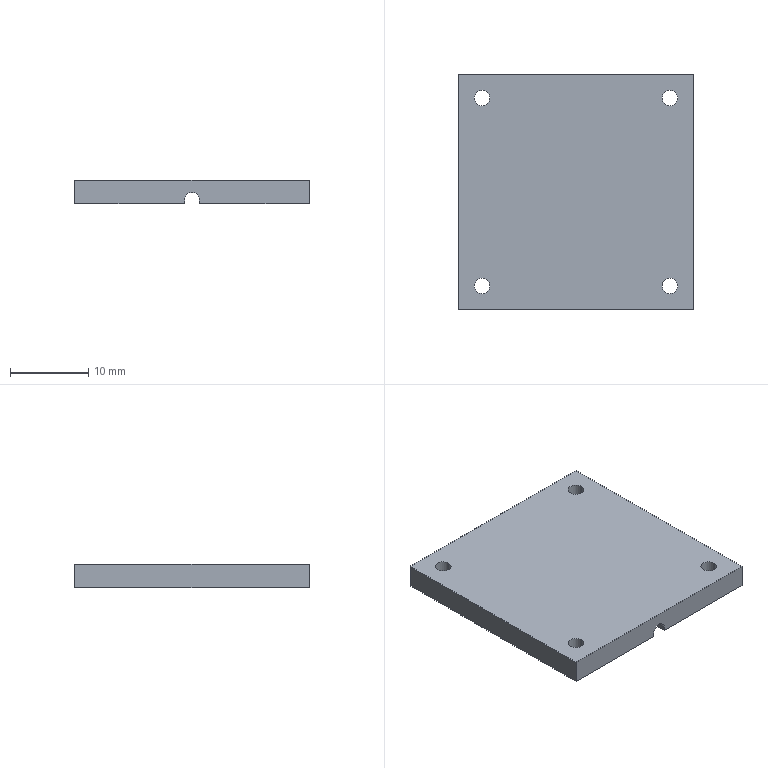Part | SolidWorks | features ICE 2, Extrusion 1 | 1 solid | 18 faces | box 30 x 30 x 3 mm | volume 2591 mm3 | cylinder 9 | plane 9 | commonest cylinder face diameters 2 x8 1.9 x1
STEP:
#1=CARTESIAN_POINT('',(-11.,-12.,0.));
#2=VERTEX_POINT('',#1);
#3=CARTESIAN_POINT('',(-13.,-12.,0.));
#4=VERTEX_POINT('',#3);
#5=CARTESIAN_POINT('',(-12.,-12.,0.));
#6=DIRECTION('',(0.,0.,-1.));
#7=DIRECTION('',(-1.,0.,0.));
#8=AXIS2_PLACEMENT_3D('',#5,#6,#7);
#9=CIRCLE('',#8,1.);
#10=EDGE_CURVE('',#2,#4,#9,.T.);
#11=ORIENTED_EDGE('',*,*,#10,.T.);
#12=CARTESIAN_POINT('',(-13.,-12.,3.));
#13=VERTEX_POINT('',#12);
#14=CARTESIAN_POINT('',(-13.,-12.,-16.));
#15=DIRECTION('',(0.,0.,1.));
#16=VECTOR('',#15,1000.);
#17=LINE('',#14,#16);
#18=EDGE_CURVE('',#4,#13,#17,.T.);
#19=ORIENTED_EDGE('',*,*,#18,.T.);
#20=CARTESIAN_POINT('',(-11.,-12.,3.));
#21=VERTEX_POINT('',#20);
#22=CARTESIAN_POINT('',(-12.,-12.,3.));
#23=DIRECTION('',(0.,0.,1.));
#24=DIRECTION('',(1.,0.,0.));
#25=AXIS2_PLACEMENT_3D('',#22,#23,#24);
#26=CIRCLE('',#25,1.);
#27=EDGE_CURVE('',#13,#21,#26,.T.);
#28=ORIENTED_EDGE('',*,*,#27,.T.);
#29=CARTESIAN_POINT('',(-11.,-12.,-16.));
#30=DIRECTION('',(0.,0.,1.));
#31=VECTOR('',#30,1000.);
#32=LINE('',#29,#31);
#33=EDGE_CURVE('',#2,#21,#32,.T.);
#34=ORIENTED_EDGE('',*,*,#33,.F.);
#35=EDGE_LOOP('',(#11,#19,#28,#34));
#36=FACE_OUTER_BOUND('',#35,.T.);
#37=CARTESIAN_POINT('',(-12.,-12.,-16.));
#38=DIRECTION('',(0.,0.,1.));
#39=DIRECTION('',(1.,0.,0.));
#40=AXIS2_PLACEMENT_3D('',#37,#38,#39);
#41=CYLINDRICAL_SURFACE('',#40,1.);
#42=ADVANCED_FACE('',(#36),#41,.F.);
#43=CARTESIAN_POINT('',(13.,-12.,0.));
#44=VERTEX_POINT('',#43);
#45=CARTESIAN_POINT('',(11.,-12.,0.));
#46=VERTEX_POINT('',#45);
#47=CARTESIAN_POINT('',(12.,-12.,0.));
#48=DIRECTION('',(0.,0.,-1.));
#49=DIRECTION('',(-1.,0.,0.));
#50=AXIS2_PLACEMENT_3D('',#47,#48,#49);
#51=CIRCLE('',#50,1.);
#52=EDGE_CURVE('',#44,#46,#51,.T.);
#53=ORIENTED_EDGE('',*,*,#52,.T.);
#54=CARTESIAN_POINT('',(11.,-12.,3.));
#55=VERTEX_POINT('',#54);
#56=CARTESIAN_POINT('',(11.,-12.,-16.));
#57=DIRECTION('',(0.,0.,1.));
#58=VECTOR('',#57,1000.);
#59=LINE('',#56,#58);
#60=EDGE_CURVE('',#46,#55,#59,.T.);
#61=ORIENTED_EDGE('',*,*,#60,.T.);
#62=CARTESIAN_POINT('',(13.,-12.,3.));
#63=VERTEX_POINT('',#62);
#64=CARTESIAN_POINT('',(12.,-12.,3.));
#65=DIRECTION('',(0.,0.,1.));
#66=DIRECTION('',(1.,0.,0.));
#67=AXIS2_PLACEMENT_3D('',#64,#65,#66);
#68=CIRCLE('',#67,1.);
#69=EDGE_CURVE('',#55,#63,#68,.T.);
#70=ORIENTED_EDGE('',*,*,#69,.T.);
#71=CARTESIAN_POINT('',(13.,-12.,-16.));
#72=DIRECTION('',(0.,0.,1.));
#73=VECTOR('',#72,1000.);
#74=LINE('',#71,#73);
#75=EDGE_CURVE('',#44,#63,#74,.T.);
#76=ORIENTED_EDGE('',*,*,#75,.F.);
#77=EDGE_LOOP('',(#53,#61,#70,#76));
#78=FACE_OUTER_BOUND('',#77,.T.);
#79=CARTESIAN_POINT('',(12.,-12.,-16.));
#80=DIRECTION('',(0.,0.,1.));
#81=DIRECTION('',(1.,0.,0.));
#82=AXIS2_PLACEMENT_3D('',#79,#80,#81);
#83=CYLINDRICAL_SURFACE('',#82,1.);
#84=ADVANCED_FACE('',(#78),#83,.F.);
#85=CARTESIAN_POINT('',(13.,12.,0.));
#86=VERTEX_POINT('',#85);
#87=CARTESIAN_POINT('',(11.,12.,0.));
#88=VERTEX_POINT('',#87);
#89=CARTESIAN_POINT('',(12.,12.,0.));
#90=DIRECTION('',(0.,0.,-1.));
#91=DIRECTION('',(-1.,0.,0.));
#92=AXIS2_PLACEMENT_3D('',#89,#90,#91);
#93=CIRCLE('',#92,1.);
#94=EDGE_CURVE('',#86,#88,#93,.T.);
#95=ORIENTED_EDGE('',*,*,#94,.T.);
#96=CARTESIAN_POINT('',(11.,12.,3.));
#97=VERTEX_POINT('',#96);
#98=CARTESIAN_POINT('',(11.,12.,-16.));
#99=DIRECTION('',(0.,0.,1.));
#100=VECTOR('',#99,1000.);
#101=LINE('',#98,#100);
#102=EDGE_CURVE('',#88,#97,#101,.T.);
#103=ORIENTED_EDGE('',*,*,#102,.T.);
#104=CARTESIAN_POINT('',(13.,12.,3.));
#105=VERTEX_POINT('',#104);
#106=CARTESIAN_POINT('',(12.,12.,3.));
#107=DIRECTION('',(0.,0.,1.));
#108=DIRECTION('',(1.,0.,0.));
#109=AXIS2_PLACEMENT_3D('',#106,#107,#108);
#110=CIRCLE('',#109,1.);
#111=EDGE_CURVE('',#97,#105,#110,.T.);
#112=ORIENTED_EDGE('',*,*,#111,.T.);
#113=CARTESIAN_POINT('',(13.,12.,-16.));
#114=DIRECTION('',(0.,0.,1.));
#115=VECTOR('',#114,1000.);
#116=LINE('',#113,#115);
#117=EDGE_CURVE('',#86,#105,#116,.T.);
#118=ORIENTED_EDGE('',*,*,#117,.F.);
#119=EDGE_LOOP('',(#95,#103,#112,#118));
#120=FACE_OUTER_BOUND('',#119,.T.);
#121=CARTESIAN_POINT('',(12.,12.,-16.));
#122=DIRECTION('',(0.,0.,1.));
#123=DIRECTION('',(1.,0.,0.));
#124=AXIS2_PLACEMENT_3D('',#121,#122,#123);
#125=CYLINDRICAL_SURFACE('',#124,1.);
#126=ADVANCED_FACE('',(#120),#125,.F.);
#127=CARTESIAN_POINT('',(-11.,12.,0.));
#128=VERTEX_POINT('',#127);
#129=CARTESIAN_POINT('',(-13.,12.,0.));
#130=VERTEX_POINT('',#129);
#131=CARTESIAN_POINT('',(-12.,12.,0.));
#132=DIRECTION('',(0.,0.,-1.));
#133=DIRECTION('',(-1.,0.,0.));
#134=AXIS2_PLACEMENT_3D('',#131,#132,#133);
#135=CIRCLE('',#134,1.);
#136=EDGE_CURVE('',#128,#130,#135,.T.);
#137=ORIENTED_EDGE('',*,*,#136,.T.);
#138=CARTESIAN_POINT('',(-13.,12.,3.));
#139=VERTEX_POINT('',#138);
#140=CARTESIAN_POINT('',(-13.,12.,-16.));
#141=DIRECTION('',(0.,0.,1.));
#142=VECTOR('',#141,1000.);
#143=LINE('',#140,#142);
#144=EDGE_CURVE('',#130,#139,#143,.T.);
#145=ORIENTED_EDGE('',*,*,#144,.T.);
#146=CARTESIAN_POINT('',(-11.,12.,3.));
#147=VERTEX_POINT('',#146);
#148=CARTESIAN_POINT('',(-12.,12.,3.));
#149=DIRECTION('',(0.,0.,1.));
#150=DIRECTION('',(1.,0.,0.));
#151=AXIS2_PLACEMENT_3D('',#148,#149,#150);
#152=CIRCLE('',#151,1.);
#153=EDGE_CURVE('',#139,#147,#152,.T.);
#154=ORIENTED_EDGE('',*,*,#153,.T.);
#155=CARTESIAN_POINT('',(-11.,12.,-16.));
#156=DIRECTION('',(0.,0.,1.));
#157=VECTOR('',#156,1000.);
#158=LINE('',#155,#157);
#159=EDGE_CURVE('',#128,#147,#158,.T.);
#160=ORIENTED_EDGE('',*,*,#159,.F.);
#161=EDGE_LOOP('',(#137,#145,#154,#160));
#162=FACE_OUTER_BOUND('',#161,.T.);
#163=CARTESIAN_POINT('',(-12.,12.,-16.));
#164=DIRECTION('',(0.,0.,1.));
#165=DIRECTION('',(1.,0.,0.));
#166=AXIS2_PLACEMENT_3D('',#163,#164,#165);
#167=CYLINDRICAL_SURFACE('',#166,1.);
#168=ADVANCED_FACE('',(#162),#167,.F.);
#169=CARTESIAN_POINT('',(0.95,15.,0.));
#170=VERTEX_POINT('',#169);
#171=CARTESIAN_POINT('',(0.95,-15.,0.));
#172=VERTEX_POINT('',#171);
#173=CARTESIAN_POINT('',(0.95,0.,0.));
#174=DIRECTION('',(0.,-1.,0.));
#175=VECTOR('',#174,1000.);
#176=LINE('',#173,#175);
#177=EDGE_CURVE('',#170,#172,#176,.T.);
#178=ORIENTED_EDGE('',*,*,#177,.F.);
#179=CARTESIAN_POINT('',(15.,15.,0.));
#180=VERTEX_POINT('',#179);
#181=CARTESIAN_POINT('',(-15.,15.,0.));
#182=DIRECTION('',(-1.,0.,0.));
#183=VECTOR('',#182,1000.);
#184=LINE('',#181,#183);
#185=EDGE_CURVE('',#180,#170,#184,.T.);
#186=ORIENTED_EDGE('',*,*,#185,.F.);
#187=CARTESIAN_POINT('',(15.,-15.,0.));
#188=VERTEX_POINT('',#187);
#189=CARTESIAN_POINT('',(15.,-15.,0.));
#190=DIRECTION('',(0.,1.,0.));
#191=VECTOR('',#190,1000.);
#192=LINE('',#189,#191);
#193=EDGE_CURVE('',#188,#180,#192,.T.);
#194=ORIENTED_EDGE('',*,*,#193,.F.);
#195=CARTESIAN_POINT('',(-15.,-15.,0.));
#196=DIRECTION('',(1.,0.,0.));
#197=VECTOR('',#196,1000.);
#198=LINE('',#195,#197);
#199=EDGE_CURVE('',#172,#188,#198,.T.);
#200=ORIENTED_EDGE('',*,*,#199,.F.);
#201=EDGE_LOOP('',(#178,#186,#194,#200));
#202=FACE_OUTER_BOUND('',#201,.T.);
#203=ORIENTED_EDGE('',*,*,#94,.F.);
#204=CARTESIAN_POINT('',(12.,12.,0.));
#205=DIRECTION('',(0.,0.,-1.));
#206=DIRECTION('',(-1.,0.,0.));
#207=AXIS2_PLACEMENT_3D('',#204,#205,#206);
#208=CIRCLE('',#207,1.);
#209=EDGE_CURVE('',#88,#86,#208,.T.);
#210=ORIENTED_EDGE('',*,*,#209,.F.);
#211=EDGE_LOOP('',(#203,#210));
#212=FACE_BOUND('',#211,.T.);
#213=ORIENTED_EDGE('',*,*,#52,.F.);
#214=CARTESIAN_POINT('',(12.,-12.,0.));
#215=DIRECTION('',(0.,0.,-1.));
#216=DIRECTION('',(-1.,0.,0.));
#217=AXIS2_PLACEMENT_3D('',#214,#215,#216);
#218=CIRCLE('',#217,1.);
#219=EDGE_CURVE('',#46,#44,#218,.T.);
#220=ORIENTED_EDGE('',*,*,#219,.F.);
#221=EDGE_LOOP('',(#213,#220));
#222=FACE_BOUND('',#221,.T.);
#223=CARTESIAN_POINT('',(0.,0.,0.));
#224=DIRECTION('',(0.,0.,-1.));
#225=DIRECTION('',(-1.,0.,0.));
#226=AXIS2_PLACEMENT_3D('',#223,#224,#225);
#227=PLANE('',#226);
#228=ADVANCED_FACE('',(#202,#212,#222),#227,.T.);
#229=ORIENTED_EDGE('',*,*,#193,.T.);
#230=CARTESIAN_POINT('',(15.,15.,3.));
#231=VERTEX_POINT('',#230);
#232=CARTESIAN_POINT('',(15.,15.,3.));
#233=DIRECTION('',(0.,0.,-1.));
#234=VECTOR('',#233,1000.);
#235=LINE('',#232,#234);
#236=EDGE_CURVE('',#231,#180,#235,.T.);
#237=ORIENTED_EDGE('',*,*,#236,.F.);
#238=CARTESIAN_POINT('',(15.,-15.,3.));
#239=VERTEX_POINT('',#238);
#240=CARTESIAN_POINT('',(15.,-15.,3.));
#241=DIRECTION('',(0.,1.,0.));
#242=VECTOR('',#241,1000.);
#243=LINE('',#240,#242);
#244=EDGE_CURVE('',#239,#231,#243,.T.);
#245=ORIENTED_EDGE('',*,*,#244,.F.);
#246=CARTESIAN_POINT('',(15.,-15.,3.));
#247=DIRECTION('',(0.,0.,-1.));
#248=VECTOR('',#247,1000.);
#249=LINE('',#246,#248);
#250=EDGE_CURVE('',#239,#188,#249,.T.);
#251=ORIENTED_EDGE('',*,*,#250,.T.);
#252=EDGE_LOOP('',(#229,#237,#245,#251));
#253=FACE_OUTER_BOUND('',#252,.T.);
#254=CARTESIAN_POINT('',(15.,-15.,3.));
#255=DIRECTION('',(-1.,0.,0.));
#256=DIRECTION('',(0.,0.,1.));
#257=AXIS2_PLACEMENT_3D('',#254,#255,#256);
#258=PLANE('',#257);
#259=ADVANCED_FACE('',(#253),#258,.F.);
#260=ORIENTED_EDGE('',*,*,#185,.T.);
#261=CARTESIAN_POINT('',(0.95,15.,0.5));
#262=VERTEX_POINT('',#261);
#263=CARTESIAN_POINT('',(0.95,15.,3.));
#264=DIRECTION('',(0.,0.,1.));
#265=VECTOR('',#264,1000.);
#266=LINE('',#263,#265);
#267=EDGE_CURVE('',#170,#262,#266,.T.);
#268=ORIENTED_EDGE('',*,*,#267,.T.);
#269=CARTESIAN_POINT('',(-0.95,15.,0.5));
#270=VERTEX_POINT('',#269);
#271=CARTESIAN_POINT('',(0.,15.,0.5));
#272=DIRECTION('',(0.,-1.,0.));
#273=DIRECTION('',(0.,0.,-1.));
#274=AXIS2_PLACEMENT_3D('',#271,#272,#273);
#275=CIRCLE('',#274,0.95);
#276=EDGE_CURVE('',#262,#270,#275,.T.);
#277=ORIENTED_EDGE('',*,*,#276,.T.);
#278=CARTESIAN_POINT('',(-0.95,15.,0.));
#279=VERTEX_POINT('',#278);
#280=CARTESIAN_POINT('',(-0.95,15.,3.));
#281=DIRECTION('',(0.,0.,-1.));
#282=VECTOR('',#281,1000.);
#283=LINE('',#280,#282);
#284=EDGE_CURVE('',#270,#279,#283,.T.);
#285=ORIENTED_EDGE('',*,*,#284,.T.);
#286=CARTESIAN_POINT('',(-15.,15.,0.));
#287=VERTEX_POINT('',#286);
#288=CARTESIAN_POINT('',(-15.,15.,0.));
#289=DIRECTION('',(-1.,0.,0.));
#290=VECTOR('',#289,1000.);
#291=LINE('',#288,#290);
#292=EDGE_CURVE('',#279,#287,#291,.T.);
#293=ORIENTED_EDGE('',*,*,#292,.T.);
#294=CARTESIAN_POINT('',(-15.,15.,3.));
#295=VERTEX_POINT('',#294);
#296=CARTESIAN_POINT('',(-15.,15.,3.));
#297=DIRECTION('',(0.,0.,-1.));
#298=VECTOR('',#297,1000.);
#299=LINE('',#296,#298);
#300=EDGE_CURVE('',#295,#287,#299,.T.);
#301=ORIENTED_EDGE('',*,*,#300,.F.);
#302=CARTESIAN_POINT('',(-15.,15.,3.));
#303=DIRECTION('',(-1.,0.,0.));
#304=VECTOR('',#303,1000.);
#305=LINE('',#302,#304);
#306=EDGE_CURVE('',#231,#295,#305,.T.);
#307=ORIENTED_EDGE('',*,*,#306,.F.);
#308=ORIENTED_EDGE('',*,*,#236,.T.);
#309=EDGE_LOOP('',(#260,#268,#277,#285,#293,#301,#307,#308));
#310=FACE_OUTER_BOUND('',#309,.T.);
#311=CARTESIAN_POINT('',(-15.,15.,3.));
#312=DIRECTION('',(0.,-1.,0.));
#313=DIRECTION('',(0.,0.,-1.));
#314=AXIS2_PLACEMENT_3D('',#311,#312,#313);
#315=PLANE('',#314);
#316=ADVANCED_FACE('',(#310),#315,.F.);
#317=CARTESIAN_POINT('',(-15.,-15.,0.));
#318=VERTEX_POINT('',#317);
#319=CARTESIAN_POINT('',(-15.,-15.,0.));
#320=DIRECTION('',(0.,-1.,0.));
#321=VECTOR('',#320,1000.);
#322=LINE('',#319,#321);
#323=EDGE_CURVE('',#287,#318,#322,.T.);
#324=ORIENTED_EDGE('',*,*,#323,.T.);
#325=CARTESIAN_POINT('',(-15.,-15.,3.));
#326=VERTEX_POINT('',#325);
#327=CARTESIAN_POINT('',(-15.,-15.,3.));
#328=DIRECTION('',(0.,0.,-1.));
#329=VECTOR('',#328,1000.);
#330=LINE('',#327,#329);
#331=EDGE_CURVE('',#326,#318,#330,.T.);
#332=ORIENTED_EDGE('',*,*,#331,.F.);
#333=CARTESIAN_POINT('',(-15.,-15.,3.));
#334=DIRECTION('',(0.,-1.,0.));
#335=VECTOR('',#334,1000.);
#336=LINE('',#333,#335);
#337=EDGE_CURVE('',#295,#326,#336,.T.);
#338=ORIENTED_EDGE('',*,*,#337,.F.);
#339=ORIENTED_EDGE('',*,*,#300,.T.);
#340=EDGE_LOOP('',(#324,#332,#338,#339));
#341=FACE_OUTER_BOUND('',#340,.T.);
#342=CARTESIAN_POINT('',(-15.,-15.,3.));
#343=DIRECTION('',(1.,0.,0.));
#344=DIRECTION('',(0.,0.,-1.));
#345=AXIS2_PLACEMENT_3D('',#342,#343,#344);
#346=PLANE('',#345);
#347=ADVANCED_FACE('',(#341),#346,.F.);
#348=CARTESIAN_POINT('',(0.95,-15.,0.5));
#349=VERTEX_POINT('',#348);
#350=CARTESIAN_POINT('',(-0.95,-15.,0.5));
#351=VERTEX_POINT('',#350);
#352=CARTESIAN_POINT('',(0.,-15.,0.5));
#353=DIRECTION('',(0.,-1.,0.));
#354=DIRECTION('',(0.,0.,-1.));
#355=AXIS2_PLACEMENT_3D('',#352,#353,#354);
#356=CIRCLE('',#355,0.95);
#357=EDGE_CURVE('',#349,#351,#356,.T.);
#358=ORIENTED_EDGE('',*,*,#357,.F.);
#359=CARTESIAN_POINT('',(0.95,-15.,0.5));
#360=DIRECTION('',(0.,0.,1.));
#361=VECTOR('',#360,1000.);
#362=LINE('',#359,#361);
#363=EDGE_CURVE('',#172,#349,#362,.T.);
#364=ORIENTED_EDGE('',*,*,#363,.F.);
#365=ORIENTED_EDGE('',*,*,#199,.T.);
#366=ORIENTED_EDGE('',*,*,#250,.F.);
#367=CARTESIAN_POINT('',(-15.,-15.,3.));
#368=DIRECTION('',(1.,0.,0.));
#369=VECTOR('',#368,1000.);
#370=LINE('',#367,#369);
#371=EDGE_CURVE('',#326,#239,#370,.T.);
#372=ORIENTED_EDGE('',*,*,#371,.F.);
#373=ORIENTED_EDGE('',*,*,#331,.T.);
#374=CARTESIAN_POINT('',(-0.95,-15.,0.));
#375=VERTEX_POINT('',#374);
#376=CARTESIAN_POINT('',(-15.,-15.,0.));
#377=DIRECTION('',(1.,0.,0.));
#378=VECTOR('',#377,1000.);
#379=LINE('',#376,#378);
#380=EDGE_CURVE('',#318,#375,#379,.T.);
#381=ORIENTED_EDGE('',*,*,#380,.T.);
#382=CARTESIAN_POINT('',(-0.95,-15.,0.));
#383=DIRECTION('',(0.,0.,-1.));
#384=VECTOR('',#383,1000.);
#385=LINE('',#382,#384);
#386=EDGE_CURVE('',#351,#375,#385,.T.);
#387=ORIENTED_EDGE('',*,*,#386,.F.);
#388=EDGE_LOOP('',(#358,#364,#365,#366,#372,#373,#381,#387));
#389=FACE_OUTER_BOUND('',#388,.T.);
#390=CARTESIAN_POINT('',(-15.,-15.,3.));
#391=DIRECTION('',(0.,1.,0.));
#392=DIRECTION('',(0.,0.,1.));
#393=AXIS2_PLACEMENT_3D('',#390,#391,#392);
#394=PLANE('',#393);
#395=ADVANCED_FACE('',(#389),#394,.F.);
#396=CARTESIAN_POINT('',(-12.,-12.,3.));
#397=DIRECTION('',(0.,0.,1.));
#398=DIRECTION('',(1.,0.,0.));
#399=AXIS2_PLACEMENT_3D('',#396,#397,#398);
#400=CIRCLE('',#399,1.);
#401=EDGE_CURVE('',#21,#13,#400,.T.);
#402=ORIENTED_EDGE('',*,*,#401,.F.);
#403=ORIENTED_EDGE('',*,*,#27,.F.);
#404=EDGE_LOOP('',(#402,#403));
#405=FACE_BOUND('',#404,.T.);
#406=CARTESIAN_POINT('',(12.,-12.,3.));
#407=DIRECTION('',(0.,0.,1.));
#408=DIRECTION('',(1.,0.,0.));
#409=AXIS2_PLACEMENT_3D('',#406,#407,#408);
#410=CIRCLE('',#409,1.);
#411=EDGE_CURVE('',#63,#55,#410,.T.);
#412=ORIENTED_EDGE('',*,*,#411,.F.);
#413=ORIENTED_EDGE('',*,*,#69,.F.);
#414=EDGE_LOOP('',(#412,#413));
#415=FACE_BOUND('',#414,.T.);
#416=CARTESIAN_POINT('',(12.,12.,3.));
#417=DIRECTION('',(0.,0.,1.));
#418=DIRECTION('',(1.,0.,0.));
#419=AXIS2_PLACEMENT_3D('',#416,#417,#418);
#420=CIRCLE('',#419,1.);
#421=EDGE_CURVE('',#105,#97,#420,.T.);
#422=ORIENTED_EDGE('',*,*,#421,.F.);
#423=ORIENTED_EDGE('',*,*,#111,.F.);
#424=EDGE_LOOP('',(#422,#423));
#425=FACE_BOUND('',#424,.T.);
#426=CARTESIAN_POINT('',(-12.,12.,3.));
#427=DIRECTION('',(0.,0.,1.));
#428=DIRECTION('',(1.,0.,0.));
#429=AXIS2_PLACEMENT_3D('',#426,#427,#428);
#430=CIRCLE('',#429,1.);
#431=EDGE_CURVE('',#147,#139,#430,.T.);
#432=ORIENTED_EDGE('',*,*,#431,.F.);
#433=ORIENTED_EDGE('',*,*,#153,.F.);
#434=EDGE_LOOP('',(#432,#433));
#435=FACE_BOUND('',#434,.T.);
#436=ORIENTED_EDGE('',*,*,#244,.T.);
#437=ORIENTED_EDGE('',*,*,#306,.T.);
#438=ORIENTED_EDGE('',*,*,#337,.T.);
#439=ORIENTED_EDGE('',*,*,#371,.T.);
#440=EDGE_LOOP('',(#436,#437,#438,#439));
#441=FACE_OUTER_BOUND('',#440,.T.);
#442=CARTESIAN_POINT('',(0.,0.,3.));
#443=DIRECTION('',(0.,0.,-1.));
#444=DIRECTION('',(-1.,0.,0.));
#445=AXIS2_PLACEMENT_3D('',#442,#443,#444);
#446=PLANE('',#445);
#447=ADVANCED_FACE('',(#405,#415,#425,#435,#441),#446,.F.);
#448=CARTESIAN_POINT('',(-0.95,0.,0.));
#449=DIRECTION('',(0.,1.,0.));
#450=VECTOR('',#449,1000.);
#451=LINE('',#448,#450);
#452=EDGE_CURVE('',#375,#279,#451,.T.);
#453=ORIENTED_EDGE('',*,*,#452,.F.);
#454=ORIENTED_EDGE('',*,*,#380,.F.);
#455=ORIENTED_EDGE('',*,*,#323,.F.);
#456=ORIENTED_EDGE('',*,*,#292,.F.);
#457=EDGE_LOOP('',(#453,#454,#455,#456));
#458=FACE_OUTER_BOUND('',#457,.T.);
#459=ORIENTED_EDGE('',*,*,#10,.F.);
#460=CARTESIAN_POINT('',(-12.,-12.,0.));
#461=DIRECTION('',(0.,0.,-1.));
#462=DIRECTION('',(-1.,0.,0.));
#463=AXIS2_PLACEMENT_3D('',#460,#461,#462);
#464=CIRCLE('',#463,1.);
#465=EDGE_CURVE('',#4,#2,#464,.T.);
#466=ORIENTED_EDGE('',*,*,#465,.F.);
#467=EDGE_LOOP('',(#459,#466));
#468=FACE_BOUND('',#467,.T.);
#469=ORIENTED_EDGE('',*,*,#136,.F.);
#470=CARTESIAN_POINT('',(-12.,12.,0.));
#471=DIRECTION('',(0.,0.,-1.));
#472=DIRECTION('',(-1.,0.,0.));
#473=AXIS2_PLACEMENT_3D('',#470,#471,#472);
#474=CIRCLE('',#473,1.);
#475=EDGE_CURVE('',#130,#128,#474,.T.);
#476=ORIENTED_EDGE('',*,*,#475,.F.);
#477=EDGE_LOOP('',(#469,#476));
#478=FACE_BOUND('',#477,.T.);
#479=CARTESIAN_POINT('',(0.,0.,0.));
#480=DIRECTION('',(0.,0.,-1.));
#481=DIRECTION('',(-1.,0.,0.));
#482=AXIS2_PLACEMENT_3D('',#479,#480,#481);
#483=PLANE('',#482);
#484=ADVANCED_FACE('',(#458,#468,#478),#483,.T.);
#485=ORIENTED_EDGE('',*,*,#144,.F.);
#486=ORIENTED_EDGE('',*,*,#475,.T.);
#487=ORIENTED_EDGE('',*,*,#159,.T.);
#488=ORIENTED_EDGE('',*,*,#431,.T.);
#489=EDGE_LOOP('',(#485,#486,#487,#488));
#490=FACE_OUTER_BOUND('',#489,.T.);
#491=CARTESIAN_POINT('',(-12.,12.,-16.));
#492=DIRECTION('',(0.,0.,1.));
#493=DIRECTION('',(1.,0.,0.));
#494=AXIS2_PLACEMENT_3D('',#491,#492,#493);
#495=CYLINDRICAL_SURFACE('',#494,1.);
#496=ADVANCED_FACE('',(#490),#495,.F.);
#497=ORIENTED_EDGE('',*,*,#102,.F.);
#498=ORIENTED_EDGE('',*,*,#209,.T.);
#499=ORIENTED_EDGE('',*,*,#117,.T.);
#500=ORIENTED_EDGE('',*,*,#421,.T.);
#501=EDGE_LOOP('',(#497,#498,#499,#500));
#502=FACE_OUTER_BOUND('',#501,.T.);
#503=CARTESIAN_POINT('',(12.,12.,-16.));
#504=DIRECTION('',(0.,0.,1.));
#505=DIRECTION('',(1.,0.,0.));
#506=AXIS2_PLACEMENT_3D('',#503,#504,#505);
#507=CYLINDRICAL_SURFACE('',#506,1.);
#508=ADVANCED_FACE('',(#502),#507,.F.);
#509=ORIENTED_EDGE('',*,*,#60,.F.);
#510=ORIENTED_EDGE('',*,*,#219,.T.);
#511=ORIENTED_EDGE('',*,*,#75,.T.);
#512=ORIENTED_EDGE('',*,*,#411,.T.);
#513=EDGE_LOOP('',(#509,#510,#511,#512));
#514=FACE_OUTER_BOUND('',#513,.T.);
#515=CARTESIAN_POINT('',(12.,-12.,-16.));
#516=DIRECTION('',(0.,0.,1.));
#517=DIRECTION('',(1.,0.,0.));
#518=AXIS2_PLACEMENT_3D('',#515,#516,#517);
#519=CYLINDRICAL_SURFACE('',#518,1.);
#520=ADVANCED_FACE('',(#514),#519,.F.);
#521=ORIENTED_EDGE('',*,*,#18,.F.);
#522=ORIENTED_EDGE('',*,*,#465,.T.);
#523=ORIENTED_EDGE('',*,*,#33,.T.);
#524=ORIENTED_EDGE('',*,*,#401,.T.);
#525=EDGE_LOOP('',(#521,#522,#523,#524));
#526=FACE_OUTER_BOUND('',#525,.T.);
#527=CARTESIAN_POINT('',(-12.,-12.,-16.));
#528=DIRECTION('',(0.,0.,1.));
#529=DIRECTION('',(1.,0.,0.));
#530=AXIS2_PLACEMENT_3D('',#527,#528,#529);
#531=CYLINDRICAL_SURFACE('',#530,1.);
#532=ADVANCED_FACE('',(#526),#531,.F.);
#533=CARTESIAN_POINT('',(0.95,27.,0.5));
#534=DIRECTION('',(0.,-1.,0.));
#535=VECTOR('',#534,1000.);
#536=LINE('',#533,#535);
#537=EDGE_CURVE('',#262,#349,#536,.T.);
#538=ORIENTED_EDGE('',*,*,#537,.T.);
#539=ORIENTED_EDGE('',*,*,#357,.T.);
#540=CARTESIAN_POINT('',(-0.95,27.,0.5));
#541=DIRECTION('',(0.,-1.,0.));
#542=VECTOR('',#541,1000.);
#543=LINE('',#540,#542);
#544=EDGE_CURVE('',#270,#351,#543,.T.);
#545=ORIENTED_EDGE('',*,*,#544,.F.);
#546=ORIENTED_EDGE('',*,*,#276,.F.);
#547=EDGE_LOOP('',(#538,#539,#545,#546));
#548=FACE_OUTER_BOUND('',#547,.T.);
#549=CARTESIAN_POINT('',(0.,27.,0.5));
#550=DIRECTION('',(0.,-1.,0.));
#551=DIRECTION('',(0.,0.,-1.));
#552=AXIS2_PLACEMENT_3D('',#549,#550,#551);
#553=CYLINDRICAL_SURFACE('',#552,0.95);
#554=ADVANCED_FACE('',(#548),#553,.F.);
#555=ORIENTED_EDGE('',*,*,#177,.T.);
#556=ORIENTED_EDGE('',*,*,#363,.T.);
#557=ORIENTED_EDGE('',*,*,#537,.F.);
#558=ORIENTED_EDGE('',*,*,#267,.F.);
#559=EDGE_LOOP('',(#555,#556,#557,#558));
#560=FACE_OUTER_BOUND('',#559,.T.);
#561=CARTESIAN_POINT('',(0.95,27.,0.5));
#562=DIRECTION('',(1.,0.,0.));
#563=DIRECTION('',(0.,0.,-1.));
#564=AXIS2_PLACEMENT_3D('',#561,#562,#563);
#565=PLANE('',#564);
#566=ADVANCED_FACE('',(#560),#565,.F.);
#567=ORIENTED_EDGE('',*,*,#544,.T.);
#568=ORIENTED_EDGE('',*,*,#386,.T.);
#569=ORIENTED_EDGE('',*,*,#452,.T.);
#570=ORIENTED_EDGE('',*,*,#284,.F.);
#571=EDGE_LOOP('',(#567,#568,#569,#570));
#572=FACE_OUTER_BOUND('',#571,.T.);
#573=CARTESIAN_POINT('',(-0.95,27.,0.));
#574=DIRECTION('',(-1.,0.,0.));
#575=DIRECTION('',(0.,0.,1.));
#576=AXIS2_PLACEMENT_3D('',#573,#574,#575);
#577=PLANE('',#576);
#578=ADVANCED_FACE('',(#572),#577,.F.);
#579=CLOSED_SHELL('',(#42,#84,#126,#168,#228,#259,#316,#347,#395,#447,#484,#496,#508,#520,#532,#554,#566,#578));
#580=MANIFOLD_SOLID_BREP('',#579);
#581=CARTESIAN_POINT('',(0.,0.,0.));
#582=DIRECTION('',(0.,0.,1.));
#583=DIRECTION('',(1.,0.,0.));
#584=AXIS2_PLACEMENT_3D('',#581,#582,#583);
#585=(LENGTH_UNIT()NAMED_UNIT(*)SI_UNIT(.MILLI.,.METRE.));
#586=UNCERTAINTY_MEASURE_WITH_UNIT(LENGTH_MEASURE(0.00001),#585,'','');
#587=(NAMED_UNIT(*)PLANE_ANGLE_UNIT()SI_UNIT($,.RADIAN.));
#588=(NAMED_UNIT(*)SI_UNIT($,.STERADIAN.)SOLID_ANGLE_UNIT());
#589=(GEOMETRIC_REPRESENTATION_CONTEXT(3)GLOBAL_UNCERTAINTY_ASSIGNED_CONTEXT((#586))GLOBAL_UNIT_ASSIGNED_CONTEXT((#585,#587,#588))REPRESENTATION_CONTEXT('',''));
#590=ADVANCED_BREP_SHAPE_REPRESENTATION('',(#580,#584),#589);